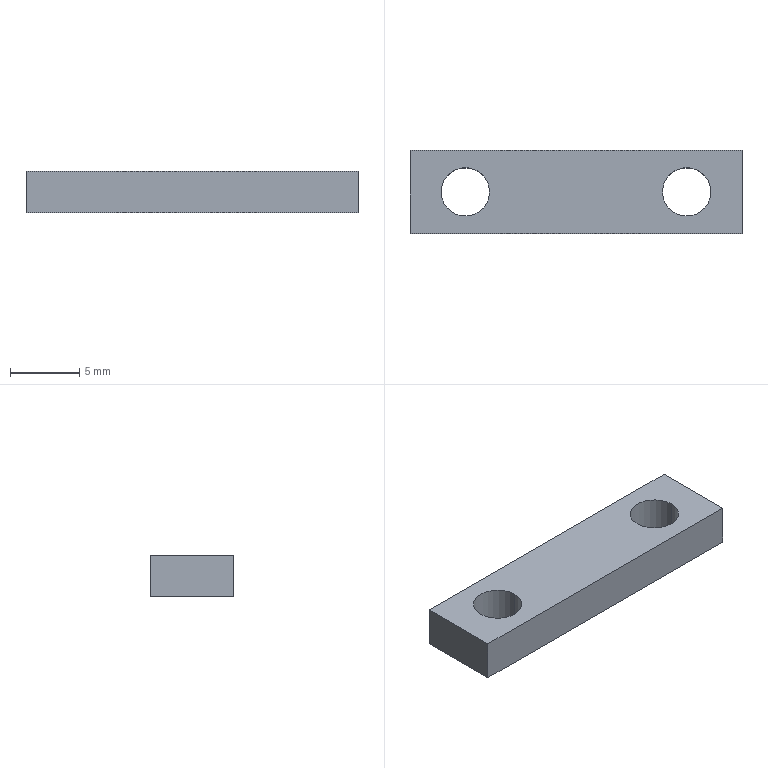Part | STEP file | Spring stop block | 1 solid | 10 faces | box 24 x 6 x 3 mm | volume 374.273 mm3 | plane 6 | cylinder 4 | commonest cylinder face diameters 3.5 x4
STEP:
#1=CARTESIAN_POINT('',(0.,0.,0.));
#2=DIRECTION('',(0.,0.,1.));
#3=DIRECTION('',(1.,0.,0.));
#4=AXIS2_PLACEMENT_3D('',#1,#2,#3);
#5=CARTESIAN_POINT('',(5.75,-3.,0.));
#6=VERTEX_POINT('',#5);
#7=CARTESIAN_POINT('',(5.75,-3.,3.));
#8=VERTEX_POINT('',#7);
#9=CARTESIAN_POINT('',(5.75,-3.,0.));
#10=DIRECTION('',(0.,0.,1.));
#11=VECTOR('',#10,1.);
#12=LINE('',#9,#11);
#13=CARTESIAN_POINT('',(4.,-3.,0.));
#14=DIRECTION('',(0.,0.,1.));
#15=DIRECTION('',(1.,0.,0.));
#16=AXIS2_PLACEMENT_3D('',#13,#14,#15);
#17=CYLINDRICAL_SURFACE('',#16,1.75);
#18=CARTESIAN_POINT('',(6.283,0.));
#19=DIRECTION('',(0.,1.));
#20=VECTOR('',#19,1.);
#21=LINE('',#18,#20);
#22=(GEOMETRIC_REPRESENTATION_CONTEXT(2)PARAMETRIC_REPRESENTATION_CONTEXT()REPRESENTATION_CONTEXT('',''));
#23=DEFINITIONAL_REPRESENTATION('',(#21),#22);
#24=PCURVE('',#17,#23);
#25=CARTESIAN_POINT('',(4.,-3.,0.));
#26=DIRECTION('',(0.,0.,1.));
#27=DIRECTION('',(1.,0.,0.));
#28=AXIS2_PLACEMENT_3D('',#25,#26,#27);
#29=CYLINDRICAL_SURFACE('',#28,1.75);
#30=CARTESIAN_POINT('',(0.,0.));
#31=DIRECTION('',(0.,1.));
#32=VECTOR('',#31,1.);
#33=LINE('',#30,#32);
#34=(GEOMETRIC_REPRESENTATION_CONTEXT(2)PARAMETRIC_REPRESENTATION_CONTEXT()REPRESENTATION_CONTEXT('',''));
#35=DEFINITIONAL_REPRESENTATION('',(#33),#34);
#36=PCURVE('',#29,#35);
#37=SURFACE_CURVE('',#12,(#24,#36),.PCURVE_S1.);
#38=EDGE_CURVE('',#6,#8,#37,.T.);
#39=ORIENTED_EDGE('',*,*,#38,.T.);
#40=CARTESIAN_POINT('',(2.25,-3.,3.));
#41=VERTEX_POINT('',#40);
#42=CARTESIAN_POINT('',(4.,-3.,3.));
#43=DIRECTION('',(0.,0.,1.));
#44=DIRECTION('',(1.,0.,0.));
#45=AXIS2_PLACEMENT_3D('',#42,#43,#44);
#46=CIRCLE('',#45,1.75);
#47=CARTESIAN_POINT('',(0.,3.));
#48=DIRECTION('',(1.,0.));
#49=VECTOR('',#48,1.);
#50=LINE('',#47,#49);
#51=(GEOMETRIC_REPRESENTATION_CONTEXT(2)PARAMETRIC_REPRESENTATION_CONTEXT()REPRESENTATION_CONTEXT('',''));
#52=DEFINITIONAL_REPRESENTATION('',(#50),#51);
#53=PCURVE('',#17,#52);
#54=CARTESIAN_POINT('',(0.,0.,3.));
#55=DIRECTION('',(0.,0.,-1.));
#56=DIRECTION('',(-1.,0.,0.));
#57=AXIS2_PLACEMENT_3D('',#54,#55,#56);
#58=PLANE('',#57);
#59=CARTESIAN_POINT('',(-5.75,-3.));
#60=CARTESIAN_POINT('',(-5.75,0.03109));
#61=CARTESIAN_POINT('',(-3.125,-1.484));
#62=CARTESIAN_POINT('',(-0.5,-3.));
#63=CARTESIAN_POINT('',(-3.125,-4.516));
#64=CARTESIAN_POINT('',(-5.75,-6.031));
#65=CARTESIAN_POINT('',(-5.75,-3.));
#66=(BOUNDED_CURVE()B_SPLINE_CURVE(2,(#59,#60,#61,#62,#63,#64,#65),.UNSPECIFIED.,.T.,.F.)B_SPLINE_CURVE_WITH_KNOTS((1,2,2,2,2,1),(-2.094,0.,2.094,4.189,6.283,8.378),.UNSPECIFIED.)CURVE()GEOMETRIC_REPRESENTATION_ITEM()RATIONAL_B_SPLINE_CURVE((1.,0.5,1.,0.5,1.,0.5,1.))REPRESENTATION_ITEM(''));
#67=(GEOMETRIC_REPRESENTATION_CONTEXT(2)PARAMETRIC_REPRESENTATION_CONTEXT()REPRESENTATION_CONTEXT('',''));
#68=DEFINITIONAL_REPRESENTATION('',(#66),#67);
#69=PCURVE('',#58,#68);
#70=SURFACE_CURVE('',#46,(#53,#69),.PCURVE_S1.);
#71=EDGE_CURVE('',#41,#8,#70,.T.);
#72=ORIENTED_EDGE('',*,*,#71,.F.);
#73=CARTESIAN_POINT('',(2.25,-3.,0.));
#74=VERTEX_POINT('',#73);
#75=CARTESIAN_POINT('',(2.25,-3.,0.));
#76=DIRECTION('',(0.,0.,1.));
#77=VECTOR('',#76,1.);
#78=LINE('',#75,#77);
#79=CARTESIAN_POINT('',(3.142,0.));
#80=DIRECTION('',(0.,1.));
#81=VECTOR('',#80,1.);
#82=LINE('',#79,#81);
#83=(GEOMETRIC_REPRESENTATION_CONTEXT(2)PARAMETRIC_REPRESENTATION_CONTEXT()REPRESENTATION_CONTEXT('',''));
#84=DEFINITIONAL_REPRESENTATION('',(#82),#83);
#85=PCURVE('',#17,#84);
#86=CARTESIAN_POINT('',(3.142,0.));
#87=DIRECTION('',(0.,1.));
#88=VECTOR('',#87,1.);
#89=LINE('',#86,#88);
#90=(GEOMETRIC_REPRESENTATION_CONTEXT(2)PARAMETRIC_REPRESENTATION_CONTEXT()REPRESENTATION_CONTEXT('',''));
#91=DEFINITIONAL_REPRESENTATION('',(#89),#90);
#92=PCURVE('',#29,#91);
#93=SURFACE_CURVE('',#78,(#85,#92),.PCURVE_S1.);
#94=EDGE_CURVE('',#74,#41,#93,.T.);
#95=ORIENTED_EDGE('',*,*,#94,.F.);
#96=CARTESIAN_POINT('',(4.,-3.,0.));
#97=DIRECTION('',(0.,0.,1.));
#98=DIRECTION('',(1.,0.,0.));
#99=AXIS2_PLACEMENT_3D('',#96,#97,#98);
#100=CIRCLE('',#99,1.75);
#101=CARTESIAN_POINT('',(0.,0.));
#102=DIRECTION('',(1.,0.));
#103=VECTOR('',#102,1.);
#104=LINE('',#101,#103);
#105=(GEOMETRIC_REPRESENTATION_CONTEXT(2)PARAMETRIC_REPRESENTATION_CONTEXT()REPRESENTATION_CONTEXT('',''));
#106=DEFINITIONAL_REPRESENTATION('',(#104),#105);
#107=PCURVE('',#17,#106);
#108=CARTESIAN_POINT('',(0.,0.,0.));
#109=DIRECTION('',(0.,0.,-1.));
#110=DIRECTION('',(-1.,0.,0.));
#111=AXIS2_PLACEMENT_3D('',#108,#109,#110);
#112=PLANE('',#111);
#113=CARTESIAN_POINT('',(-5.75,-3.));
#114=CARTESIAN_POINT('',(-5.75,0.03109));
#115=CARTESIAN_POINT('',(-3.125,-1.484));
#116=CARTESIAN_POINT('',(-0.5,-3.));
#117=CARTESIAN_POINT('',(-3.125,-4.516));
#118=CARTESIAN_POINT('',(-5.75,-6.031));
#119=CARTESIAN_POINT('',(-5.75,-3.));
#120=(BOUNDED_CURVE()B_SPLINE_CURVE(2,(#113,#114,#115,#116,#117,#118,#119),.UNSPECIFIED.,.T.,.F.)B_SPLINE_CURVE_WITH_KNOTS((1,2,2,2,2,1),(-2.094,0.,2.094,4.189,6.283,8.378),.UNSPECIFIED.)CURVE()GEOMETRIC_REPRESENTATION_ITEM()RATIONAL_B_SPLINE_CURVE((1.,0.5,1.,0.5,1.,0.5,1.))REPRESENTATION_ITEM(''));
#121=(GEOMETRIC_REPRESENTATION_CONTEXT(2)PARAMETRIC_REPRESENTATION_CONTEXT()REPRESENTATION_CONTEXT('',''));
#122=DEFINITIONAL_REPRESENTATION('',(#120),#121);
#123=PCURVE('',#112,#122);
#124=SURFACE_CURVE('',#100,(#107,#123),.PCURVE_S1.);
#125=EDGE_CURVE('',#74,#6,#124,.T.);
#126=ORIENTED_EDGE('',*,*,#125,.T.);
#127=EDGE_LOOP('',(#39,#72,#95,#126));
#128=FACE_BOUND('',#127,.F.);
#129=ADVANCED_FACE('',(#128),#17,.F.);
#130=CARTESIAN_POINT('',(21.75,-3.,0.));
#131=VERTEX_POINT('',#130);
#132=CARTESIAN_POINT('',(21.75,-3.,3.));
#133=VERTEX_POINT('',#132);
#134=CARTESIAN_POINT('',(21.75,-3.,0.));
#135=DIRECTION('',(0.,0.,1.));
#136=VECTOR('',#135,1.);
#137=LINE('',#134,#136);
#138=CARTESIAN_POINT('',(20.,-3.,0.));
#139=DIRECTION('',(0.,0.,1.));
#140=DIRECTION('',(1.,0.,0.));
#141=AXIS2_PLACEMENT_3D('',#138,#139,#140);
#142=CYLINDRICAL_SURFACE('',#141,1.75);
#143=CARTESIAN_POINT('',(6.283,0.));
#144=DIRECTION('',(0.,1.));
#145=VECTOR('',#144,1.);
#146=LINE('',#143,#145);
#147=(GEOMETRIC_REPRESENTATION_CONTEXT(2)PARAMETRIC_REPRESENTATION_CONTEXT()REPRESENTATION_CONTEXT('',''));
#148=DEFINITIONAL_REPRESENTATION('',(#146),#147);
#149=PCURVE('',#142,#148);
#150=CARTESIAN_POINT('',(20.,-3.,0.));
#151=DIRECTION('',(0.,0.,1.));
#152=DIRECTION('',(1.,0.,0.));
#153=AXIS2_PLACEMENT_3D('',#150,#151,#152);
#154=CYLINDRICAL_SURFACE('',#153,1.75);
#155=CARTESIAN_POINT('',(0.,0.));
#156=DIRECTION('',(0.,1.));
#157=VECTOR('',#156,1.);
#158=LINE('',#155,#157);
#159=(GEOMETRIC_REPRESENTATION_CONTEXT(2)PARAMETRIC_REPRESENTATION_CONTEXT()REPRESENTATION_CONTEXT('',''));
#160=DEFINITIONAL_REPRESENTATION('',(#158),#159);
#161=PCURVE('',#154,#160);
#162=SURFACE_CURVE('',#137,(#149,#161),.PCURVE_S1.);
#163=EDGE_CURVE('',#131,#133,#162,.T.);
#164=ORIENTED_EDGE('',*,*,#163,.T.);
#165=CARTESIAN_POINT('',(18.25,-3.,3.));
#166=VERTEX_POINT('',#165);
#167=CARTESIAN_POINT('',(20.,-3.,3.));
#168=DIRECTION('',(0.,0.,1.));
#169=DIRECTION('',(1.,0.,0.));
#170=AXIS2_PLACEMENT_3D('',#167,#168,#169);
#171=CIRCLE('',#170,1.75);
#172=CARTESIAN_POINT('',(0.,3.));
#173=DIRECTION('',(1.,0.));
#174=VECTOR('',#173,1.);
#175=LINE('',#172,#174);
#176=(GEOMETRIC_REPRESENTATION_CONTEXT(2)PARAMETRIC_REPRESENTATION_CONTEXT()REPRESENTATION_CONTEXT('',''));
#177=DEFINITIONAL_REPRESENTATION('',(#175),#176);
#178=PCURVE('',#142,#177);
#179=CARTESIAN_POINT('',(-21.75,-3.));
#180=CARTESIAN_POINT('',(-21.75,0.03109));
#181=CARTESIAN_POINT('',(-19.125,-1.484));
#182=CARTESIAN_POINT('',(-16.5,-3.));
#183=CARTESIAN_POINT('',(-19.125,-4.516));
#184=CARTESIAN_POINT('',(-21.75,-6.031));
#185=CARTESIAN_POINT('',(-21.75,-3.));
#186=(BOUNDED_CURVE()B_SPLINE_CURVE(2,(#179,#180,#181,#182,#183,#184,#185),.UNSPECIFIED.,.T.,.F.)B_SPLINE_CURVE_WITH_KNOTS((1,2,2,2,2,1),(-2.094,0.,2.094,4.189,6.283,8.378),.UNSPECIFIED.)CURVE()GEOMETRIC_REPRESENTATION_ITEM()RATIONAL_B_SPLINE_CURVE((1.,0.5,1.,0.5,1.,0.5,1.))REPRESENTATION_ITEM(''));
#187=(GEOMETRIC_REPRESENTATION_CONTEXT(2)PARAMETRIC_REPRESENTATION_CONTEXT()REPRESENTATION_CONTEXT('',''));
#188=DEFINITIONAL_REPRESENTATION('',(#186),#187);
#189=PCURVE('',#58,#188);
#190=SURFACE_CURVE('',#171,(#178,#189),.PCURVE_S1.);
#191=EDGE_CURVE('',#166,#133,#190,.T.);
#192=ORIENTED_EDGE('',*,*,#191,.F.);
#193=CARTESIAN_POINT('',(18.25,-3.,0.));
#194=VERTEX_POINT('',#193);
#195=CARTESIAN_POINT('',(18.25,-3.,0.));
#196=DIRECTION('',(0.,0.,1.));
#197=VECTOR('',#196,1.);
#198=LINE('',#195,#197);
#199=CARTESIAN_POINT('',(3.142,0.));
#200=DIRECTION('',(0.,1.));
#201=VECTOR('',#200,1.);
#202=LINE('',#199,#201);
#203=(GEOMETRIC_REPRESENTATION_CONTEXT(2)PARAMETRIC_REPRESENTATION_CONTEXT()REPRESENTATION_CONTEXT('',''));
#204=DEFINITIONAL_REPRESENTATION('',(#202),#203);
#205=PCURVE('',#142,#204);
#206=CARTESIAN_POINT('',(3.142,0.));
#207=DIRECTION('',(0.,1.));
#208=VECTOR('',#207,1.);
#209=LINE('',#206,#208);
#210=(GEOMETRIC_REPRESENTATION_CONTEXT(2)PARAMETRIC_REPRESENTATION_CONTEXT()REPRESENTATION_CONTEXT('',''));
#211=DEFINITIONAL_REPRESENTATION('',(#209),#210);
#212=PCURVE('',#154,#211);
#213=SURFACE_CURVE('',#198,(#205,#212),.PCURVE_S1.);
#214=EDGE_CURVE('',#194,#166,#213,.T.);
#215=ORIENTED_EDGE('',*,*,#214,.F.);
#216=CARTESIAN_POINT('',(20.,-3.,0.));
#217=DIRECTION('',(0.,0.,1.));
#218=DIRECTION('',(1.,0.,0.));
#219=AXIS2_PLACEMENT_3D('',#216,#217,#218);
#220=CIRCLE('',#219,1.75);
#221=CARTESIAN_POINT('',(0.,0.));
#222=DIRECTION('',(1.,0.));
#223=VECTOR('',#222,1.);
#224=LINE('',#221,#223);
#225=(GEOMETRIC_REPRESENTATION_CONTEXT(2)PARAMETRIC_REPRESENTATION_CONTEXT()REPRESENTATION_CONTEXT('',''));
#226=DEFINITIONAL_REPRESENTATION('',(#224),#225);
#227=PCURVE('',#142,#226);
#228=CARTESIAN_POINT('',(-21.75,-3.));
#229=CARTESIAN_POINT('',(-21.75,0.03109));
#230=CARTESIAN_POINT('',(-19.125,-1.484));
#231=CARTESIAN_POINT('',(-16.5,-3.));
#232=CARTESIAN_POINT('',(-19.125,-4.516));
#233=CARTESIAN_POINT('',(-21.75,-6.031));
#234=CARTESIAN_POINT('',(-21.75,-3.));
#235=(BOUNDED_CURVE()B_SPLINE_CURVE(2,(#228,#229,#230,#231,#232,#233,#234),.UNSPECIFIED.,.T.,.F.)B_SPLINE_CURVE_WITH_KNOTS((1,2,2,2,2,1),(-2.094,0.,2.094,4.189,6.283,8.378),.UNSPECIFIED.)CURVE()GEOMETRIC_REPRESENTATION_ITEM()RATIONAL_B_SPLINE_CURVE((1.,0.5,1.,0.5,1.,0.5,1.))REPRESENTATION_ITEM(''));
#236=(GEOMETRIC_REPRESENTATION_CONTEXT(2)PARAMETRIC_REPRESENTATION_CONTEXT()REPRESENTATION_CONTEXT('',''));
#237=DEFINITIONAL_REPRESENTATION('',(#235),#236);
#238=PCURVE('',#112,#237);
#239=SURFACE_CURVE('',#220,(#227,#238),.PCURVE_S1.);
#240=EDGE_CURVE('',#194,#131,#239,.T.);
#241=ORIENTED_EDGE('',*,*,#240,.T.);
#242=EDGE_LOOP('',(#164,#192,#215,#241));
#243=FACE_BOUND('',#242,.F.);
#244=ADVANCED_FACE('',(#243),#142,.F.);
#245=CARTESIAN_POINT('',(0.,0.,0.));
#246=VERTEX_POINT('',#245);
#247=CARTESIAN_POINT('',(0.,-6.,0.));
#248=VERTEX_POINT('',#247);
#249=CARTESIAN_POINT('',(0.,-6.,0.));
#250=DIRECTION('',(0.,-1.,0.));
#251=VECTOR('',#250,1.);
#252=LINE('',#249,#251);
#253=CARTESIAN_POINT('',(0.,-6.,3.));
#254=DIRECTION('',(1.,0.,0.));
#255=DIRECTION('',(0.,0.,-1.));
#256=AXIS2_PLACEMENT_3D('',#253,#254,#255);
#257=PLANE('',#256);
#258=CARTESIAN_POINT('',(3.,0.));
#259=DIRECTION('',(0.,-1.));
#260=VECTOR('',#259,1.);
#261=LINE('',#258,#260);
#262=(GEOMETRIC_REPRESENTATION_CONTEXT(2)PARAMETRIC_REPRESENTATION_CONTEXT()REPRESENTATION_CONTEXT('',''));
#263=DEFINITIONAL_REPRESENTATION('',(#261),#262);
#264=PCURVE('',#257,#263);
#265=CARTESIAN_POINT('',(0.,-6.));
#266=DIRECTION('',(0.,-1.));
#267=VECTOR('',#266,1.);
#268=LINE('',#265,#267);
#269=(GEOMETRIC_REPRESENTATION_CONTEXT(2)PARAMETRIC_REPRESENTATION_CONTEXT()REPRESENTATION_CONTEXT('',''));
#270=DEFINITIONAL_REPRESENTATION('',(#268),#269);
#271=PCURVE('',#112,#270);
#272=SURFACE_CURVE('',#252,(#264,#271),.PCURVE_S1.);
#273=EDGE_CURVE('',#246,#248,#272,.T.);
#274=ORIENTED_EDGE('',*,*,#273,.T.);
#275=CARTESIAN_POINT('',(0.,-6.,3.));
#276=VERTEX_POINT('',#275);
#277=CARTESIAN_POINT('',(0.,-6.,3.));
#278=DIRECTION('',(0.,0.,-1.));
#279=VECTOR('',#278,1.);
#280=LINE('',#277,#279);
#281=CARTESIAN_POINT('',(0.,0.));
#282=DIRECTION('',(1.,0.));
#283=VECTOR('',#282,1.);
#284=LINE('',#281,#283);
#285=(GEOMETRIC_REPRESENTATION_CONTEXT(2)PARAMETRIC_REPRESENTATION_CONTEXT()REPRESENTATION_CONTEXT('',''));
#286=DEFINITIONAL_REPRESENTATION('',(#284),#285);
#287=PCURVE('',#257,#286);
#288=CARTESIAN_POINT('',(0.,-6.,3.));
#289=DIRECTION('',(0.,1.,0.));
#290=DIRECTION('',(0.,0.,1.));
#291=AXIS2_PLACEMENT_3D('',#288,#289,#290);
#292=PLANE('',#291);
#293=CARTESIAN_POINT('',(0.,0.));
#294=DIRECTION('',(-1.,0.));
#295=VECTOR('',#294,1.);
#296=LINE('',#293,#295);
#297=(GEOMETRIC_REPRESENTATION_CONTEXT(2)PARAMETRIC_REPRESENTATION_CONTEXT()REPRESENTATION_CONTEXT('',''));
#298=DEFINITIONAL_REPRESENTATION('',(#296),#297);
#299=PCURVE('',#292,#298);
#300=SURFACE_CURVE('',#280,(#287,#299),.PCURVE_S1.);
#301=EDGE_CURVE('',#276,#248,#300,.T.);
#302=ORIENTED_EDGE('',*,*,#301,.F.);
#303=CARTESIAN_POINT('',(0.,0.,3.));
#304=VERTEX_POINT('',#303);
#305=CARTESIAN_POINT('',(0.,-6.,3.));
#306=DIRECTION('',(0.,-1.,0.));
#307=VECTOR('',#306,1.);
#308=LINE('',#305,#307);
#309=CARTESIAN_POINT('',(0.,0.));
#310=DIRECTION('',(0.,-1.));
#311=VECTOR('',#310,1.);
#312=LINE('',#309,#311);
#313=(GEOMETRIC_REPRESENTATION_CONTEXT(2)PARAMETRIC_REPRESENTATION_CONTEXT()REPRESENTATION_CONTEXT('',''));
#314=DEFINITIONAL_REPRESENTATION('',(#312),#313);
#315=PCURVE('',#257,#314);
#316=CARTESIAN_POINT('',(0.,-6.));
#317=DIRECTION('',(0.,-1.));
#318=VECTOR('',#317,1.);
#319=LINE('',#316,#318);
#320=(GEOMETRIC_REPRESENTATION_CONTEXT(2)PARAMETRIC_REPRESENTATION_CONTEXT()REPRESENTATION_CONTEXT('',''));
#321=DEFINITIONAL_REPRESENTATION('',(#319),#320);
#322=PCURVE('',#58,#321);
#323=SURFACE_CURVE('',#308,(#315,#322),.PCURVE_S1.);
#324=EDGE_CURVE('',#304,#276,#323,.T.);
#325=ORIENTED_EDGE('',*,*,#324,.F.);
#326=CARTESIAN_POINT('',(0.,0.,3.));
#327=DIRECTION('',(0.,0.,-1.));
#328=VECTOR('',#327,1.);
#329=LINE('',#326,#328);
#330=CARTESIAN_POINT('',(0.,6.));
#331=DIRECTION('',(1.,0.));
#332=VECTOR('',#331,1.);
#333=LINE('',#330,#332);
#334=(GEOMETRIC_REPRESENTATION_CONTEXT(2)PARAMETRIC_REPRESENTATION_CONTEXT()REPRESENTATION_CONTEXT('',''));
#335=DEFINITIONAL_REPRESENTATION('',(#333),#334);
#336=PCURVE('',#257,#335);
#337=CARTESIAN_POINT('',(0.,0.,3.));
#338=DIRECTION('',(0.,-1.,0.));
#339=DIRECTION('',(0.,0.,-1.));
#340=AXIS2_PLACEMENT_3D('',#337,#338,#339);
#341=PLANE('',#340);
#342=CARTESIAN_POINT('',(0.,0.));
#343=DIRECTION('',(1.,0.));
#344=VECTOR('',#343,1.);
#345=LINE('',#342,#344);
#346=(GEOMETRIC_REPRESENTATION_CONTEXT(2)PARAMETRIC_REPRESENTATION_CONTEXT()REPRESENTATION_CONTEXT('',''));
#347=DEFINITIONAL_REPRESENTATION('',(#345),#346);
#348=PCURVE('',#341,#347);
#349=SURFACE_CURVE('',#329,(#336,#348),.PCURVE_S1.);
#350=EDGE_CURVE('',#304,#246,#349,.T.);
#351=ORIENTED_EDGE('',*,*,#350,.T.);
#352=EDGE_LOOP('',(#274,#302,#325,#351));
#353=FACE_BOUND('',#352,.T.);
#354=ADVANCED_FACE('',(#353),#257,.F.);
#355=CARTESIAN_POINT('',(24.,-6.,0.));
#356=VERTEX_POINT('',#355);
#357=CARTESIAN_POINT('',(0.,-6.,0.));
#358=DIRECTION('',(1.,0.,0.));
#359=VECTOR('',#358,1.);
#360=LINE('',#357,#359);
#361=CARTESIAN_POINT('',(-3.,0.));
#362=DIRECTION('',(0.,1.));
#363=VECTOR('',#362,1.);
#364=LINE('',#361,#363);
#365=(GEOMETRIC_REPRESENTATION_CONTEXT(2)PARAMETRIC_REPRESENTATION_CONTEXT()REPRESENTATION_CONTEXT('',''));
#366=DEFINITIONAL_REPRESENTATION('',(#364),#365);
#367=PCURVE('',#292,#366);
#368=CARTESIAN_POINT('',(0.,-6.));
#369=DIRECTION('',(-1.,0.));
#370=VECTOR('',#369,1.);
#371=LINE('',#368,#370);
#372=(GEOMETRIC_REPRESENTATION_CONTEXT(2)PARAMETRIC_REPRESENTATION_CONTEXT()REPRESENTATION_CONTEXT('',''));
#373=DEFINITIONAL_REPRESENTATION('',(#371),#372);
#374=PCURVE('',#112,#373);
#375=SURFACE_CURVE('',#360,(#367,#374),.PCURVE_S1.);
#376=EDGE_CURVE('',#248,#356,#375,.T.);
#377=ORIENTED_EDGE('',*,*,#376,.T.);
#378=CARTESIAN_POINT('',(24.,-6.,3.));
#379=VERTEX_POINT('',#378);
#380=CARTESIAN_POINT('',(24.,-6.,3.));
#381=DIRECTION('',(0.,0.,-1.));
#382=VECTOR('',#381,1.);
#383=LINE('',#380,#382);
#384=CARTESIAN_POINT('',(0.,24.));
#385=DIRECTION('',(-1.,0.));
#386=VECTOR('',#385,1.);
#387=LINE('',#384,#386);
#388=(GEOMETRIC_REPRESENTATION_CONTEXT(2)PARAMETRIC_REPRESENTATION_CONTEXT()REPRESENTATION_CONTEXT('',''));
#389=DEFINITIONAL_REPRESENTATION('',(#387),#388);
#390=PCURVE('',#292,#389);
#391=CARTESIAN_POINT('',(24.,-6.,3.));
#392=DIRECTION('',(-1.,0.,0.));
#393=DIRECTION('',(0.,0.,1.));
#394=AXIS2_PLACEMENT_3D('',#391,#392,#393);
#395=PLANE('',#394);
#396=CARTESIAN_POINT('',(0.,0.));
#397=DIRECTION('',(-1.,0.));
#398=VECTOR('',#397,1.);
#399=LINE('',#396,#398);
#400=(GEOMETRIC_REPRESENTATION_CONTEXT(2)PARAMETRIC_REPRESENTATION_CONTEXT()REPRESENTATION_CONTEXT('',''));
#401=DEFINITIONAL_REPRESENTATION('',(#399),#400);
#402=PCURVE('',#395,#401);
#403=SURFACE_CURVE('',#383,(#390,#402),.PCURVE_S1.);
#404=EDGE_CURVE('',#379,#356,#403,.T.);
#405=ORIENTED_EDGE('',*,*,#404,.F.);
#406=CARTESIAN_POINT('',(0.,-6.,3.));
#407=DIRECTION('',(1.,0.,0.));
#408=VECTOR('',#407,1.);
#409=LINE('',#406,#408);
#410=CARTESIAN_POINT('',(0.,0.));
#411=DIRECTION('',(0.,1.));
#412=VECTOR('',#411,1.);
#413=LINE('',#410,#412);
#414=(GEOMETRIC_REPRESENTATION_CONTEXT(2)PARAMETRIC_REPRESENTATION_CONTEXT()REPRESENTATION_CONTEXT('',''));
#415=DEFINITIONAL_REPRESENTATION('',(#413),#414);
#416=PCURVE('',#292,#415);
#417=CARTESIAN_POINT('',(0.,-6.));
#418=DIRECTION('',(-1.,0.));
#419=VECTOR('',#418,1.);
#420=LINE('',#417,#419);
#421=(GEOMETRIC_REPRESENTATION_CONTEXT(2)PARAMETRIC_REPRESENTATION_CONTEXT()REPRESENTATION_CONTEXT('',''));
#422=DEFINITIONAL_REPRESENTATION('',(#420),#421);
#423=PCURVE('',#58,#422);
#424=SURFACE_CURVE('',#409,(#416,#423),.PCURVE_S1.);
#425=EDGE_CURVE('',#276,#379,#424,.T.);
#426=ORIENTED_EDGE('',*,*,#425,.F.);
#427=ORIENTED_EDGE('',*,*,#301,.T.);
#428=EDGE_LOOP('',(#377,#405,#426,#427));
#429=FACE_BOUND('',#428,.T.);
#430=ADVANCED_FACE('',(#429),#292,.F.);
#431=CARTESIAN_POINT('',(24.,0.,0.));
#432=VERTEX_POINT('',#431);
#433=CARTESIAN_POINT('',(24.,-6.,0.));
#434=DIRECTION('',(0.,1.,0.));
#435=VECTOR('',#434,1.);
#436=LINE('',#433,#435);
#437=CARTESIAN_POINT('',(-3.,0.));
#438=DIRECTION('',(0.,1.));
#439=VECTOR('',#438,1.);
#440=LINE('',#437,#439);
#441=(GEOMETRIC_REPRESENTATION_CONTEXT(2)PARAMETRIC_REPRESENTATION_CONTEXT()REPRESENTATION_CONTEXT('',''));
#442=DEFINITIONAL_REPRESENTATION('',(#440),#441);
#443=PCURVE('',#395,#442);
#444=CARTESIAN_POINT('',(-24.,-6.));
#445=DIRECTION('',(0.,1.));
#446=VECTOR('',#445,1.);
#447=LINE('',#444,#446);
#448=(GEOMETRIC_REPRESENTATION_CONTEXT(2)PARAMETRIC_REPRESENTATION_CONTEXT()REPRESENTATION_CONTEXT('',''));
#449=DEFINITIONAL_REPRESENTATION('',(#447),#448);
#450=PCURVE('',#112,#449);
#451=SURFACE_CURVE('',#436,(#443,#450),.PCURVE_S1.);
#452=EDGE_CURVE('',#356,#432,#451,.T.);
#453=ORIENTED_EDGE('',*,*,#452,.T.);
#454=CARTESIAN_POINT('',(24.,0.,3.));
#455=VERTEX_POINT('',#454);
#456=CARTESIAN_POINT('',(24.,0.,3.));
#457=DIRECTION('',(0.,0.,-1.));
#458=VECTOR('',#457,1.);
#459=LINE('',#456,#458);
#460=CARTESIAN_POINT('',(0.,6.));
#461=DIRECTION('',(-1.,0.));
#462=VECTOR('',#461,1.);
#463=LINE('',#460,#462);
#464=(GEOMETRIC_REPRESENTATION_CONTEXT(2)PARAMETRIC_REPRESENTATION_CONTEXT()REPRESENTATION_CONTEXT('',''));
#465=DEFINITIONAL_REPRESENTATION('',(#463),#464);
#466=PCURVE('',#395,#465);
#467=CARTESIAN_POINT('',(0.,24.));
#468=DIRECTION('',(1.,0.));
#469=VECTOR('',#468,1.);
#470=LINE('',#467,#469);
#471=(GEOMETRIC_REPRESENTATION_CONTEXT(2)PARAMETRIC_REPRESENTATION_CONTEXT()REPRESENTATION_CONTEXT('',''));
#472=DEFINITIONAL_REPRESENTATION('',(#470),#471);
#473=PCURVE('',#341,#472);
#474=SURFACE_CURVE('',#459,(#466,#473),.PCURVE_S1.);
#475=EDGE_CURVE('',#455,#432,#474,.T.);
#476=ORIENTED_EDGE('',*,*,#475,.F.);
#477=CARTESIAN_POINT('',(24.,-6.,3.));
#478=DIRECTION('',(0.,1.,0.));
#479=VECTOR('',#478,1.);
#480=LINE('',#477,#479);
#481=CARTESIAN_POINT('',(0.,0.));
#482=DIRECTION('',(0.,1.));
#483=VECTOR('',#482,1.);
#484=LINE('',#481,#483);
#485=(GEOMETRIC_REPRESENTATION_CONTEXT(2)PARAMETRIC_REPRESENTATION_CONTEXT()REPRESENTATION_CONTEXT('',''));
#486=DEFINITIONAL_REPRESENTATION('',(#484),#485);
#487=PCURVE('',#395,#486);
#488=CARTESIAN_POINT('',(-24.,-6.));
#489=DIRECTION('',(0.,1.));
#490=VECTOR('',#489,1.);
#491=LINE('',#488,#490);
#492=(GEOMETRIC_REPRESENTATION_CONTEXT(2)PARAMETRIC_REPRESENTATION_CONTEXT()REPRESENTATION_CONTEXT('',''));
#493=DEFINITIONAL_REPRESENTATION('',(#491),#492);
#494=PCURVE('',#58,#493);
#495=SURFACE_CURVE('',#480,(#487,#494),.PCURVE_S1.);
#496=EDGE_CURVE('',#379,#455,#495,.T.);
#497=ORIENTED_EDGE('',*,*,#496,.F.);
#498=ORIENTED_EDGE('',*,*,#404,.T.);
#499=EDGE_LOOP('',(#453,#476,#497,#498));
#500=FACE_BOUND('',#499,.T.);
#501=ADVANCED_FACE('',(#500),#395,.F.);
#502=CARTESIAN_POINT('',(0.,0.,0.));
#503=DIRECTION('',(-1.,0.,0.));
#504=VECTOR('',#503,1.);
#505=LINE('',#502,#504);
#506=CARTESIAN_POINT('',(3.,0.));
#507=DIRECTION('',(0.,-1.));
#508=VECTOR('',#507,1.);
#509=LINE('',#506,#508);
#510=(GEOMETRIC_REPRESENTATION_CONTEXT(2)PARAMETRIC_REPRESENTATION_CONTEXT()REPRESENTATION_CONTEXT('',''));
#511=DEFINITIONAL_REPRESENTATION('',(#509),#510);
#512=PCURVE('',#341,#511);
#513=CARTESIAN_POINT('',(0.,0.));
#514=DIRECTION('',(1.,0.));
#515=VECTOR('',#514,1.);
#516=LINE('',#513,#515);
#517=(GEOMETRIC_REPRESENTATION_CONTEXT(2)PARAMETRIC_REPRESENTATION_CONTEXT()REPRESENTATION_CONTEXT('',''));
#518=DEFINITIONAL_REPRESENTATION('',(#516),#517);
#519=PCURVE('',#112,#518);
#520=SURFACE_CURVE('',#505,(#512,#519),.PCURVE_S1.);
#521=EDGE_CURVE('',#432,#246,#520,.T.);
#522=ORIENTED_EDGE('',*,*,#521,.T.);
#523=ORIENTED_EDGE('',*,*,#350,.F.);
#524=CARTESIAN_POINT('',(0.,0.,3.));
#525=DIRECTION('',(-1.,0.,0.));
#526=VECTOR('',#525,1.);
#527=LINE('',#524,#526);
#528=CARTESIAN_POINT('',(0.,0.));
#529=DIRECTION('',(0.,-1.));
#530=VECTOR('',#529,1.);
#531=LINE('',#528,#530);
#532=(GEOMETRIC_REPRESENTATION_CONTEXT(2)PARAMETRIC_REPRESENTATION_CONTEXT()REPRESENTATION_CONTEXT('',''));
#533=DEFINITIONAL_REPRESENTATION('',(#531),#532);
#534=PCURVE('',#341,#533);
#535=CARTESIAN_POINT('',(0.,0.));
#536=DIRECTION('',(1.,0.));
#537=VECTOR('',#536,1.);
#538=LINE('',#535,#537);
#539=(GEOMETRIC_REPRESENTATION_CONTEXT(2)PARAMETRIC_REPRESENTATION_CONTEXT()REPRESENTATION_CONTEXT('',''));
#540=DEFINITIONAL_REPRESENTATION('',(#538),#539);
#541=PCURVE('',#58,#540);
#542=SURFACE_CURVE('',#527,(#534,#541),.PCURVE_S1.);
#543=EDGE_CURVE('',#455,#304,#542,.T.);
#544=ORIENTED_EDGE('',*,*,#543,.F.);
#545=ORIENTED_EDGE('',*,*,#475,.T.);
#546=EDGE_LOOP('',(#522,#523,#544,#545));
#547=FACE_BOUND('',#546,.T.);
#548=ADVANCED_FACE('',(#547),#341,.F.);
#549=CARTESIAN_POINT('',(4.,-3.,3.));
#550=DIRECTION('',(0.,0.,1.));
#551=DIRECTION('',(1.,0.,0.));
#552=AXIS2_PLACEMENT_3D('',#549,#550,#551);
#553=CIRCLE('',#552,1.75);
#554=CARTESIAN_POINT('',(-5.75,-3.));
#555=CARTESIAN_POINT('',(-5.75,0.03109));
#556=CARTESIAN_POINT('',(-3.125,-1.484));
#557=CARTESIAN_POINT('',(-0.5,-3.));
#558=CARTESIAN_POINT('',(-3.125,-4.516));
#559=CARTESIAN_POINT('',(-5.75,-6.031));
#560=CARTESIAN_POINT('',(-5.75,-3.));
#561=(BOUNDED_CURVE()B_SPLINE_CURVE(2,(#554,#555,#556,#557,#558,#559,#560),.UNSPECIFIED.,.T.,.F.)B_SPLINE_CURVE_WITH_KNOTS((1,2,2,2,2,1),(-2.094,0.,2.094,4.189,6.283,8.378),.UNSPECIFIED.)CURVE()GEOMETRIC_REPRESENTATION_ITEM()RATIONAL_B_SPLINE_CURVE((1.,0.5,1.,0.5,1.,0.5,1.))REPRESENTATION_ITEM(''));
#562=(GEOMETRIC_REPRESENTATION_CONTEXT(2)PARAMETRIC_REPRESENTATION_CONTEXT()REPRESENTATION_CONTEXT('',''));
#563=DEFINITIONAL_REPRESENTATION('',(#561),#562);
#564=PCURVE('',#58,#563);
#565=CARTESIAN_POINT('',(0.,3.));
#566=DIRECTION('',(1.,0.));
#567=VECTOR('',#566,1.);
#568=LINE('',#565,#567);
#569=(GEOMETRIC_REPRESENTATION_CONTEXT(2)PARAMETRIC_REPRESENTATION_CONTEXT()REPRESENTATION_CONTEXT('',''));
#570=DEFINITIONAL_REPRESENTATION('',(#568),#569);
#571=PCURVE('',#29,#570);
#572=SURFACE_CURVE('',#553,(#564,#571),.PCURVE_S1.);
#573=EDGE_CURVE('',#8,#41,#572,.T.);
#574=ORIENTED_EDGE('',*,*,#573,.F.);
#575=ORIENTED_EDGE('',*,*,#71,.F.);
#576=EDGE_LOOP('',(#574,#575));
#577=FACE_BOUND('',#576,.T.);
#578=CARTESIAN_POINT('',(20.,-3.,3.));
#579=DIRECTION('',(0.,0.,1.));
#580=DIRECTION('',(1.,0.,0.));
#581=AXIS2_PLACEMENT_3D('',#578,#579,#580);
#582=CIRCLE('',#581,1.75);
#583=CARTESIAN_POINT('',(-21.75,-3.));
#584=CARTESIAN_POINT('',(-21.75,0.03109));
#585=CARTESIAN_POINT('',(-19.125,-1.484));
#586=CARTESIAN_POINT('',(-16.5,-3.));
#587=CARTESIAN_POINT('',(-19.125,-4.516));
#588=CARTESIAN_POINT('',(-21.75,-6.031));
#589=CARTESIAN_POINT('',(-21.75,-3.));
#590=(BOUNDED_CURVE()B_SPLINE_CURVE(2,(#583,#584,#585,#586,#587,#588,#589),.UNSPECIFIED.,.T.,.F.)B_SPLINE_CURVE_WITH_KNOTS((1,2,2,2,2,1),(-2.094,0.,2.094,4.189,6.283,8.378),.UNSPECIFIED.)CURVE()GEOMETRIC_REPRESENTATION_ITEM()RATIONAL_B_SPLINE_CURVE((1.,0.5,1.,0.5,1.,0.5,1.))REPRESENTATION_ITEM(''));
#591=(GEOMETRIC_REPRESENTATION_CONTEXT(2)PARAMETRIC_REPRESENTATION_CONTEXT()REPRESENTATION_CONTEXT('',''));
#592=DEFINITIONAL_REPRESENTATION('',(#590),#591);
#593=PCURVE('',#58,#592);
#594=CARTESIAN_POINT('',(0.,3.));
#595=DIRECTION('',(1.,0.));
#596=VECTOR('',#595,1.);
#597=LINE('',#594,#596);
#598=(GEOMETRIC_REPRESENTATION_CONTEXT(2)PARAMETRIC_REPRESENTATION_CONTEXT()REPRESENTATION_CONTEXT('',''));
#599=DEFINITIONAL_REPRESENTATION('',(#597),#598);
#600=PCURVE('',#154,#599);
#601=SURFACE_CURVE('',#582,(#593,#600),.PCURVE_S1.);
#602=EDGE_CURVE('',#133,#166,#601,.T.);
#603=ORIENTED_EDGE('',*,*,#602,.F.);
#604=ORIENTED_EDGE('',*,*,#191,.F.);
#605=EDGE_LOOP('',(#603,#604));
#606=FACE_BOUND('',#605,.T.);
#607=ORIENTED_EDGE('',*,*,#324,.T.);
#608=ORIENTED_EDGE('',*,*,#425,.T.);
#609=ORIENTED_EDGE('',*,*,#496,.T.);
#610=ORIENTED_EDGE('',*,*,#543,.T.);
#611=EDGE_LOOP('',(#607,#608,#609,#610));
#612=FACE_BOUND('',#611,.T.);
#613=ADVANCED_FACE('',(#577,#606,#612),#58,.F.);
#614=CARTESIAN_POINT('',(4.,-3.,0.));
#615=DIRECTION('',(0.,0.,1.));
#616=DIRECTION('',(1.,0.,0.));
#617=AXIS2_PLACEMENT_3D('',#614,#615,#616);
#618=CIRCLE('',#617,1.75);
#619=CARTESIAN_POINT('',(-5.75,-3.));
#620=CARTESIAN_POINT('',(-5.75,0.03109));
#621=CARTESIAN_POINT('',(-3.125,-1.484));
#622=CARTESIAN_POINT('',(-0.5,-3.));
#623=CARTESIAN_POINT('',(-3.125,-4.516));
#624=CARTESIAN_POINT('',(-5.75,-6.031));
#625=CARTESIAN_POINT('',(-5.75,-3.));
#626=(BOUNDED_CURVE()B_SPLINE_CURVE(2,(#619,#620,#621,#622,#623,#624,#625),.UNSPECIFIED.,.T.,.F.)B_SPLINE_CURVE_WITH_KNOTS((1,2,2,2,2,1),(-2.094,0.,2.094,4.189,6.283,8.378),.UNSPECIFIED.)CURVE()GEOMETRIC_REPRESENTATION_ITEM()RATIONAL_B_SPLINE_CURVE((1.,0.5,1.,0.5,1.,0.5,1.))REPRESENTATION_ITEM(''));
#627=(GEOMETRIC_REPRESENTATION_CONTEXT(2)PARAMETRIC_REPRESENTATION_CONTEXT()REPRESENTATION_CONTEXT('',''));
#628=DEFINITIONAL_REPRESENTATION('',(#626),#627);
#629=PCURVE('',#112,#628);
#630=CARTESIAN_POINT('',(0.,0.));
#631=DIRECTION('',(1.,0.));
#632=VECTOR('',#631,1.);
#633=LINE('',#630,#632);
#634=(GEOMETRIC_REPRESENTATION_CONTEXT(2)PARAMETRIC_REPRESENTATION_CONTEXT()REPRESENTATION_CONTEXT('',''));
#635=DEFINITIONAL_REPRESENTATION('',(#633),#634);
#636=PCURVE('',#29,#635);
#637=SURFACE_CURVE('',#618,(#629,#636),.PCURVE_S1.);
#638=EDGE_CURVE('',#6,#74,#637,.T.);
#639=ORIENTED_EDGE('',*,*,#638,.T.);
#640=ORIENTED_EDGE('',*,*,#125,.T.);
#641=EDGE_LOOP('',(#639,#640));
#642=FACE_BOUND('',#641,.T.);
#643=CARTESIAN_POINT('',(20.,-3.,0.));
#644=DIRECTION('',(0.,0.,1.));
#645=DIRECTION('',(1.,0.,0.));
#646=AXIS2_PLACEMENT_3D('',#643,#644,#645);
#647=CIRCLE('',#646,1.75);
#648=CARTESIAN_POINT('',(-21.75,-3.));
#649=CARTESIAN_POINT('',(-21.75,0.03109));
#650=CARTESIAN_POINT('',(-19.125,-1.484));
#651=CARTESIAN_POINT('',(-16.5,-3.));
#652=CARTESIAN_POINT('',(-19.125,-4.516));
#653=CARTESIAN_POINT('',(-21.75,-6.031));
#654=CARTESIAN_POINT('',(-21.75,-3.));
#655=(BOUNDED_CURVE()B_SPLINE_CURVE(2,(#648,#649,#650,#651,#652,#653,#654),.UNSPECIFIED.,.T.,.F.)B_SPLINE_CURVE_WITH_KNOTS((1,2,2,2,2,1),(-2.094,0.,2.094,4.189,6.283,8.378),.UNSPECIFIED.)CURVE()GEOMETRIC_REPRESENTATION_ITEM()RATIONAL_B_SPLINE_CURVE((1.,0.5,1.,0.5,1.,0.5,1.))REPRESENTATION_ITEM(''));
#656=(GEOMETRIC_REPRESENTATION_CONTEXT(2)PARAMETRIC_REPRESENTATION_CONTEXT()REPRESENTATION_CONTEXT('',''));
#657=DEFINITIONAL_REPRESENTATION('',(#655),#656);
#658=PCURVE('',#112,#657);
#659=CARTESIAN_POINT('',(0.,0.));
#660=DIRECTION('',(1.,0.));
#661=VECTOR('',#660,1.);
#662=LINE('',#659,#661);
#663=(GEOMETRIC_REPRESENTATION_CONTEXT(2)PARAMETRIC_REPRESENTATION_CONTEXT()REPRESENTATION_CONTEXT('',''));
#664=DEFINITIONAL_REPRESENTATION('',(#662),#663);
#665=PCURVE('',#154,#664);
#666=SURFACE_CURVE('',#647,(#658,#665),.PCURVE_S1.);
#667=EDGE_CURVE('',#131,#194,#666,.T.);
#668=ORIENTED_EDGE('',*,*,#667,.T.);
#669=ORIENTED_EDGE('',*,*,#240,.T.);
#670=EDGE_LOOP('',(#668,#669));
#671=FACE_BOUND('',#670,.T.);
#672=ORIENTED_EDGE('',*,*,#273,.F.);
#673=ORIENTED_EDGE('',*,*,#521,.F.);
#674=ORIENTED_EDGE('',*,*,#452,.F.);
#675=ORIENTED_EDGE('',*,*,#376,.F.);
#676=EDGE_LOOP('',(#672,#673,#674,#675));
#677=FACE_BOUND('',#676,.T.);
#678=ADVANCED_FACE('',(#642,#671,#677),#112,.T.);
#679=ORIENTED_EDGE('',*,*,#602,.F.);
#680=ORIENTED_EDGE('',*,*,#163,.F.);
#681=ORIENTED_EDGE('',*,*,#667,.T.);
#682=ORIENTED_EDGE('',*,*,#214,.T.);
#683=EDGE_LOOP('',(#679,#680,#681,#682));
#684=FACE_BOUND('',#683,.F.);
#685=ADVANCED_FACE('',(#684),#154,.F.);
#686=ORIENTED_EDGE('',*,*,#573,.F.);
#687=ORIENTED_EDGE('',*,*,#38,.F.);
#688=ORIENTED_EDGE('',*,*,#638,.T.);
#689=ORIENTED_EDGE('',*,*,#94,.T.);
#690=EDGE_LOOP('',(#686,#687,#688,#689));
#691=FACE_BOUND('',#690,.F.);
#692=ADVANCED_FACE('',(#691),#29,.F.);
#693=CLOSED_SHELL('',(#129,#244,#354,#430,#501,#548,#613,#678,#685,#692));
#694=MANIFOLD_SOLID_BREP('',#693);
#695=(LENGTH_UNIT()NAMED_UNIT(*)SI_UNIT(.MILLI.,.METRE.));
#696=UNCERTAINTY_MEASURE_WITH_UNIT(LENGTH_MEASURE(0.0000001),#695,'','');
#697=(NAMED_UNIT(*)PLANE_ANGLE_UNIT()SI_UNIT($,.RADIAN.));
#698=(NAMED_UNIT(*)SI_UNIT($,.STERADIAN.)SOLID_ANGLE_UNIT());
#699=(GEOMETRIC_REPRESENTATION_CONTEXT(3)GLOBAL_UNCERTAINTY_ASSIGNED_CONTEXT((#696))GLOBAL_UNIT_ASSIGNED_CONTEXT((#695,#697,#698))REPRESENTATION_CONTEXT('',''));
#700=ADVANCED_BREP_SHAPE_REPRESENTATION('',(#4,#694),#699);